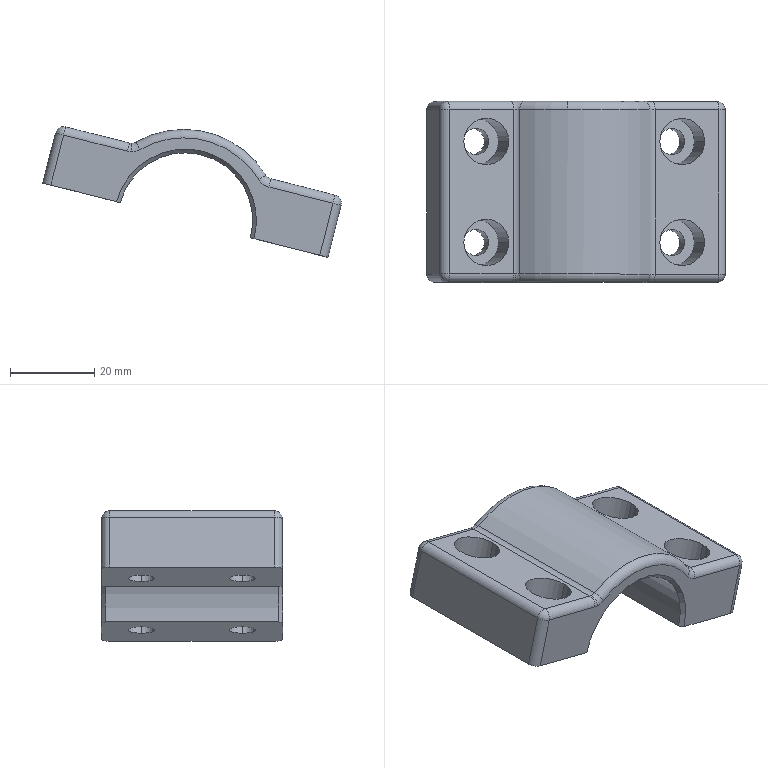Part | SolidWorks | features BaseBody 1 | 1 solid | 58 faces | box 70.928 x 43 x 31.032 mm | volume 28593 mm3 | cylinder 31 | plane 12 | torus 8 | sphere 4 | cone 3 | commonest cylinder face diameters 4 x12 6.2 x8 11 x8 32 x2 46 x1